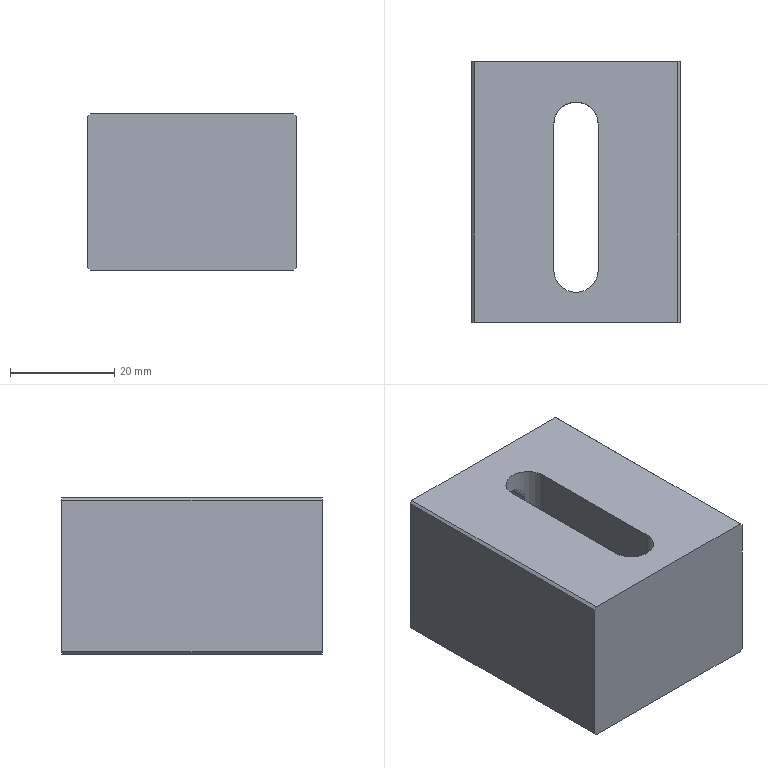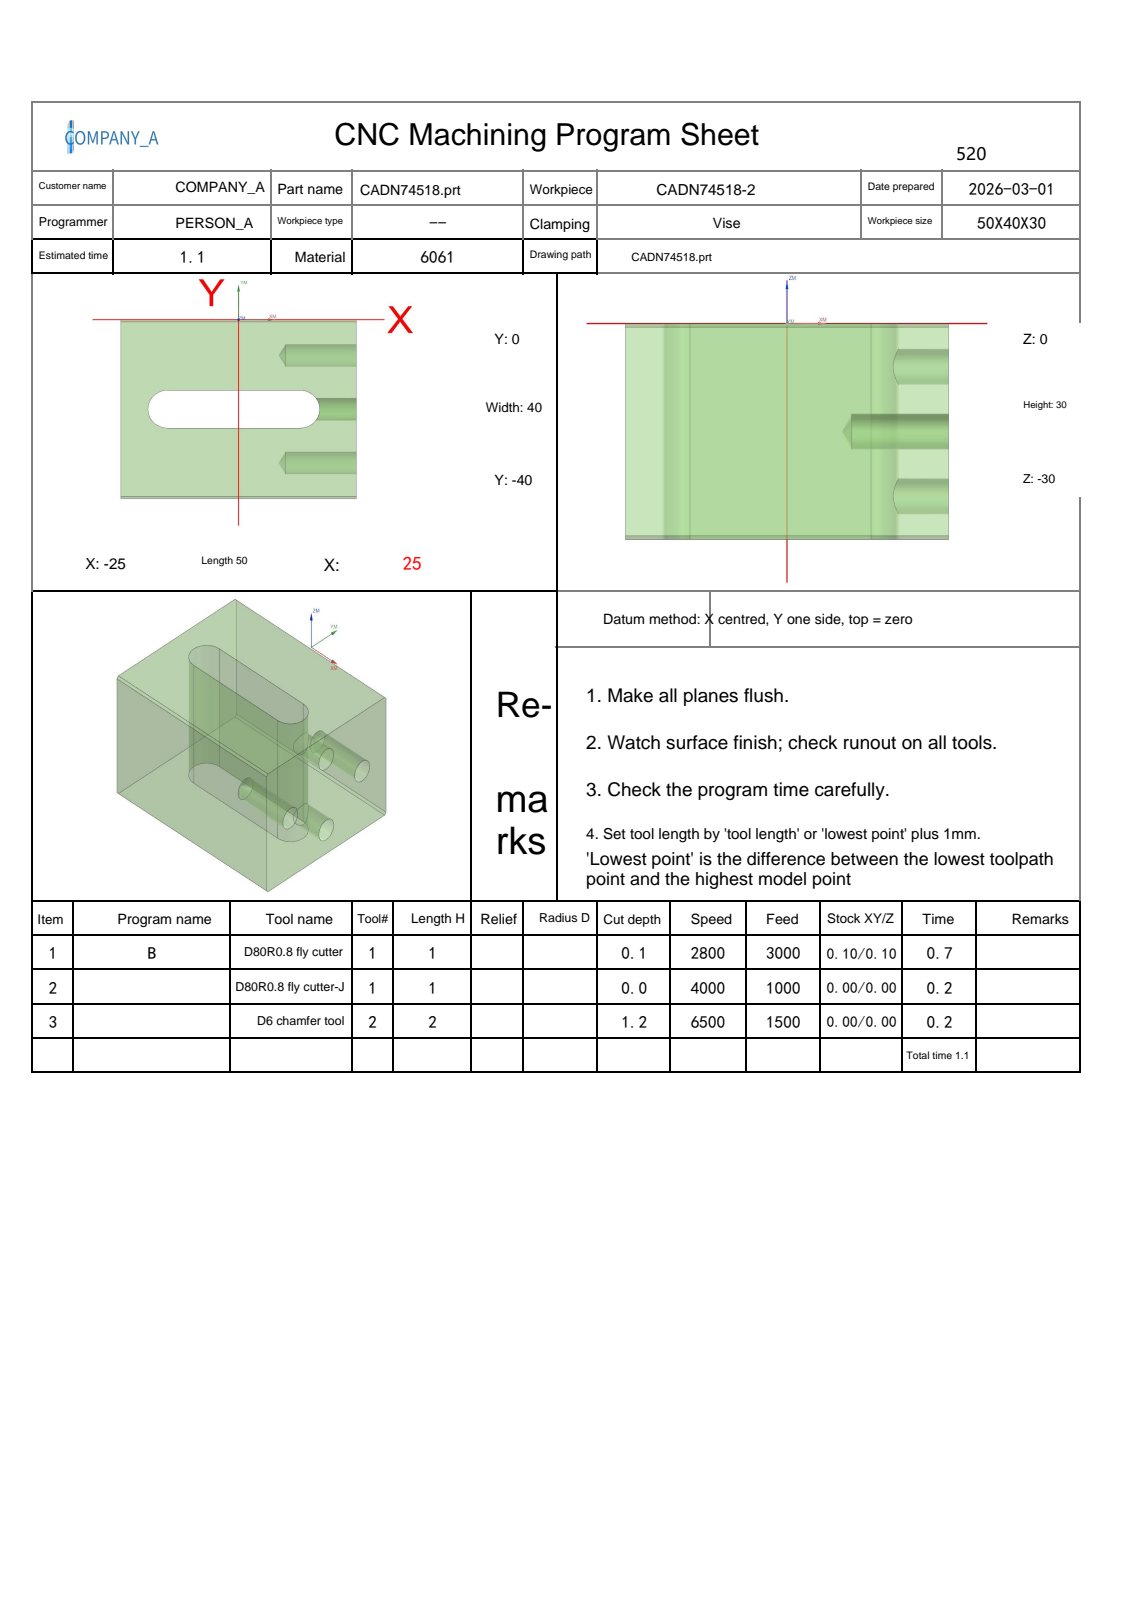NC program | NX | posted by the shop | part box 40 x 50 x 30 mm
Whole program:
%
O0001
(Machine time: 1.61 MIN)
(===Total Tool:2===)
(T1=D80R0.8 fly cutter D=80.  R=0.8  D-  H01 Z=0.    )
(T2=D6 chamfer tool   D=6.   R=0.   D-  H02 Z=-1.2  )
G80 G90 G17 G49 G40
G91 G28 Z0
M01
N1 T01 M06
(D80R0.8 fly cutter D=80. R=0.8 H=01 ce=0.10 di=0.10)
G00 G90 G54 X-77.097 Y-20. M03 S2800
G43 H01 Z50.
M08
Z6.011
G01 Z4.011 F3000.
X-65.097
X65.097
X77.097
Z6.011
G00 X-77.097
Z5.522
G01 Z3.522
X-65.097
X65.097
X77.097
Z5.522
G00 X-77.097
Z5.033
G01 Z3.033
X-65.097
X65.097
X77.097
Z5.033
G00 X-77.097
Z4.544
G01 Z2.544
X-65.097
X65.097
X77.097
Z4.544
G00 Z50.
X-77.097
Z4.056
G01 Z2.056
X-65.097
X65.097
X77.097
Z4.056
G00 Z50.
X-77.097
Z3.567
G01 Z1.567
X-65.097
X65.097
X77.097
Z3.567
G00 Z50.
X-77.097
Z3.078
G01 Z1.078
X-65.097
X65.097
X77.097
Z3.078
G00 Z50.
X-77.097
Z2.589
G01 Z.589
X-65.097
X65.097
X77.097
Z2.589
G00 Z50.
X-77.097
Z2.1
G01 Z.1
X-65.097
X65.097
X77.097
Z2.1
G00 Z50.
G91 G28 Z0.0
M05
M09
G91 G28 Z0.0
M01
N2 T01 M06
(D80R0.8 fly cutter-J D=80. R=0.8 H=01 ce=0.00 di=0.00)
G00 G90 G54 X-76.999 Y-20. M03 S4000
G43 H01 Z50.
M08
Z2.
G01 Z0.0 F1000.
X-64.999
X64.999
X76.999
Z2.
G00 Z50.
G91 G28 Z0.0
M05
M09
G91 G28 Z0.0
M01
N3 T02 M06
(D6 chamfer tool D=6. R=0. H=02 ce=0.00 di=0.00)
G00 G90 G54 X25.99 Y.292 M03 S6500
G43 H02 Z50.
M08
Z.13
G01 Z-1.2 F1500.
G03 X25.915 Y-.048 I1.907 J-.601
G01 X25.905 Y-.102
X25.928 Y-.151
X25.966 Y-.241
X26. Y-.5
Y-39.5
X25.966 Y-39.759
X25.928 Y-39.849
X25.905 Y-39.898
X25.915 Y-39.952
G03 X25.99 Y-40.292 I1.983 J.261
G01 Z.13
G00 Z10.
X-25.99
Z.13
G01 Z-1.2
G03 X-25.915 Y-39.952 I-1.907 J.601
G01 X-25.905 Y-39.898
X-25.928 Y-39.849
X-25.966 Y-39.759
X-26. Y-39.5
Y-.5
X-25.966 Y-.241
X-25.928 Y-.151
X-25.905 Y-.102
X-25.915 Y-.048
G03 X-25.99 Y.292 I-1.983 J-.261
G01 Z.13
G00 Z10.
X-1.386 Y-23.023
Z.172
G01 Z-1.2
G03 X-1.1 Y-23.223 I1.286 J1.532
G01 X-1.054 Y-23.253
X-1. Y-23.25
X13.
G03 X16.25 Y-20. I0.0 J3.25
X13. Y-16.75 I-3.25 J0.0
G01 X-15.
G03 X-18.25 Y-20. I0.0 J-3.25
X-15. Y-23.25 I3.25 J0.0
G01 X-1.
X-.946 Y-23.253
X-.9 Y-23.223
G03 X-.614 Y-23.023 I-1. J1.732
G01 Z.172
G00 Z50.
G00 G90 X28.963 Y-41.9 M03 S6500
Z50.
Z.3
G01 Z-1.2 F1500.
G03 X27.763 Y-40.7 I-1.2 J0.0
G01 X-27.763
G03 X-28.963 Y-41.9 I0.0 J-1.2
G01 Z.3
G00 Z50.
Y1.9
Z.3
G01 Z-1.2
G03 X-27.763 Y.7 I1.2 J0.0
G01 X27.763
G03 X28.963 Y1.9 I0.0 J1.2
G01 Z.3
G00 Z50.
M05
M09
G91 G28 Z0.0
G91 G28 Y0.0
M30
%